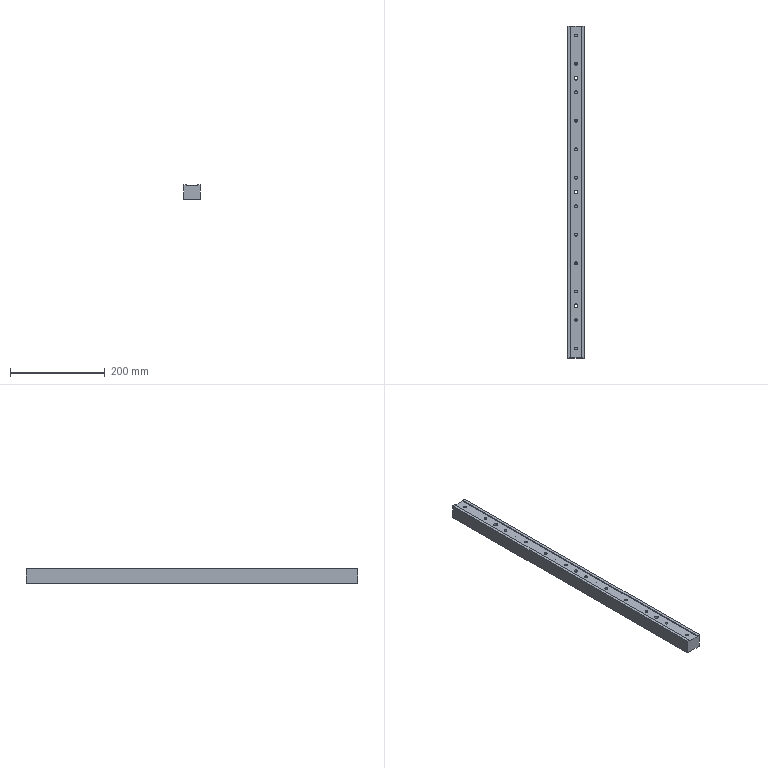Part | STEP file | Tube feed_id1466_x_t | 1 solid | 67 faces | box 35 x 700 x 30 mm | volume 688178 mm3 | cone 24 | plane 22 | cylinder 21 | commonest cylinder face diameters 5 x12 6.8 x6 8 x3